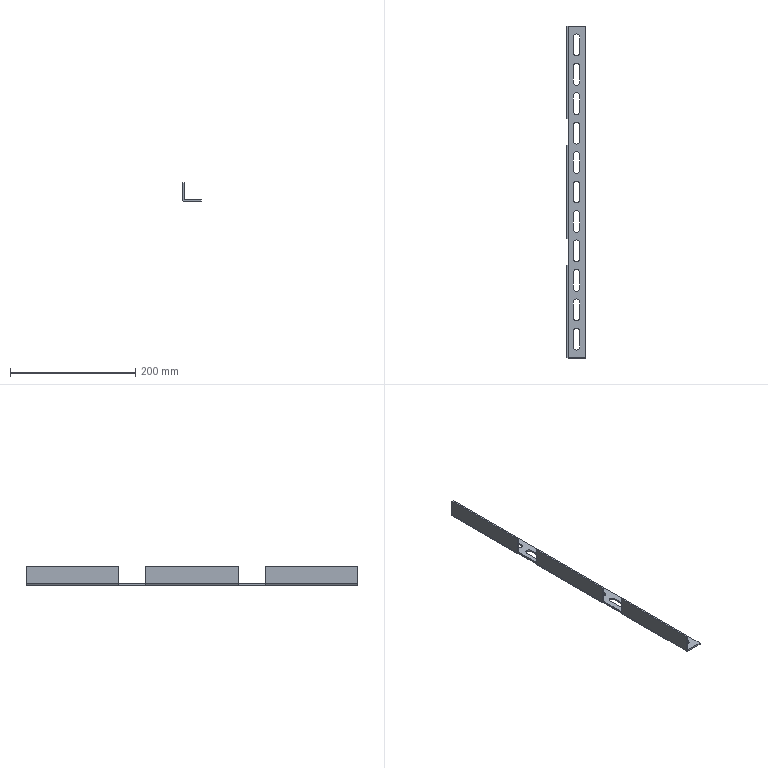Part | SolidWorks | features ICE 2, EdgeFlange 1, FlatPattern 1, LPattern 1, SMBaseFlange 1, SheetMetal 1 | 1 solid | 85 faces | box 30 x 530 x 30 mm | volume 60196 mm3 | plane 50 | cylinder 35 | commonest cylinder face diameters 10 x33 0.2 x1 5.2 x1